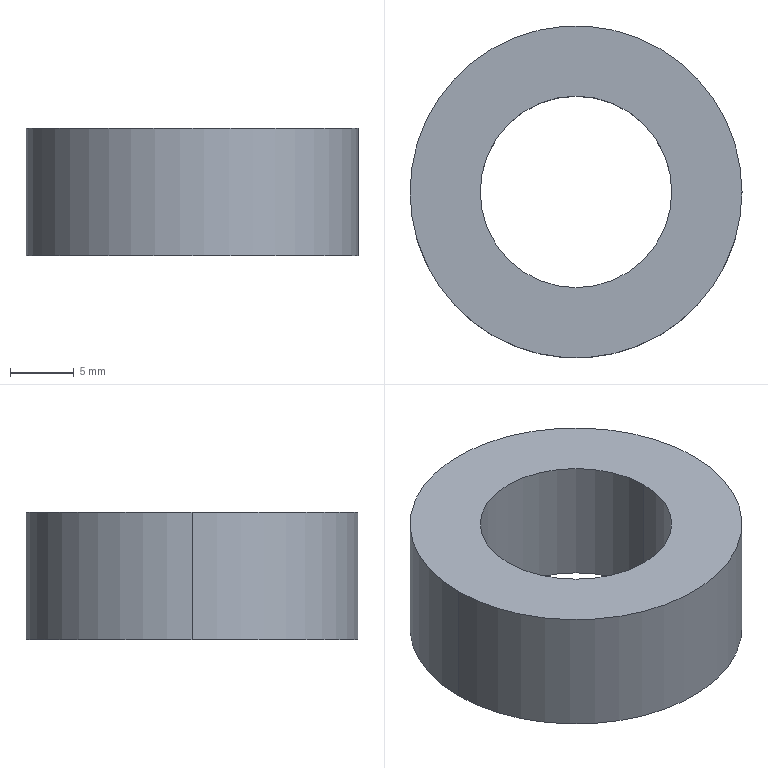Part | SolidWorks | features Extrusion 1 | 1 solid | 6 faces | box 26 x 26 x 10 mm | volume 3542 mm3 | cylinder 4 | plane 2 | commonest cylinder face diameters 15 x2 26 x2
STEP:
#1=CARTESIAN_POINT('',(-7.5,0.,5.));
#2=VERTEX_POINT('',#1);
#3=CARTESIAN_POINT('',(7.5,0.,5.));
#4=VERTEX_POINT('',#3);
#5=CARTESIAN_POINT('',(0.,0.,5.));
#6=DIRECTION('',(0.,0.,1.));
#7=DIRECTION('',(1.,0.,0.));
#8=AXIS2_PLACEMENT_3D('',#5,#6,#7);
#9=CIRCLE('',#8,7.5);
#10=EDGE_CURVE('',#2,#4,#9,.T.);
#11=ORIENTED_EDGE('',*,*,#10,.T.);
#12=CARTESIAN_POINT('',(7.5,0.,-5.));
#13=VERTEX_POINT('',#12);
#14=CARTESIAN_POINT('',(7.5,0.,5.));
#15=DIRECTION('',(0.,0.,-1.));
#16=VECTOR('',#15,1000.);
#17=LINE('',#14,#16);
#18=EDGE_CURVE('',#4,#13,#17,.T.);
#19=ORIENTED_EDGE('',*,*,#18,.T.);
#20=CARTESIAN_POINT('',(-7.5,0.,-5.));
#21=VERTEX_POINT('',#20);
#22=CARTESIAN_POINT('',(0.,0.,-5.));
#23=DIRECTION('',(0.,0.,1.));
#24=DIRECTION('',(1.,0.,0.));
#25=AXIS2_PLACEMENT_3D('',#22,#23,#24);
#26=CIRCLE('',#25,7.5);
#27=EDGE_CURVE('',#21,#13,#26,.T.);
#28=ORIENTED_EDGE('',*,*,#27,.F.);
#29=CARTESIAN_POINT('',(-7.5,0.,5.));
#30=DIRECTION('',(0.,0.,-1.));
#31=VECTOR('',#30,1000.);
#32=LINE('',#29,#31);
#33=EDGE_CURVE('',#2,#21,#32,.T.);
#34=ORIENTED_EDGE('',*,*,#33,.F.);
#35=EDGE_LOOP('',(#11,#19,#28,#34));
#36=FACE_OUTER_BOUND('',#35,.T.);
#37=CARTESIAN_POINT('',(0.,0.,5.));
#38=DIRECTION('',(0.,0.,-1.));
#39=DIRECTION('',(-1.,0.,0.));
#40=AXIS2_PLACEMENT_3D('',#37,#38,#39);
#41=CYLINDRICAL_SURFACE('',#40,7.5);
#42=ADVANCED_FACE('',(#36),#41,.F.);
#43=CARTESIAN_POINT('',(13.,0.,5.));
#44=VERTEX_POINT('',#43);
#45=CARTESIAN_POINT('',(-13.,0.,5.));
#46=VERTEX_POINT('',#45);
#47=CARTESIAN_POINT('',(0.,0.,5.));
#48=DIRECTION('',(0.,0.,1.));
#49=DIRECTION('',(1.,0.,0.));
#50=AXIS2_PLACEMENT_3D('',#47,#48,#49);
#51=CIRCLE('',#50,13.);
#52=EDGE_CURVE('',#44,#46,#51,.T.);
#53=ORIENTED_EDGE('',*,*,#52,.F.);
#54=CARTESIAN_POINT('',(13.,0.,-5.));
#55=VERTEX_POINT('',#54);
#56=CARTESIAN_POINT('',(13.,0.,5.));
#57=DIRECTION('',(0.,0.,-1.));
#58=VECTOR('',#57,1000.);
#59=LINE('',#56,#58);
#60=EDGE_CURVE('',#44,#55,#59,.T.);
#61=ORIENTED_EDGE('',*,*,#60,.T.);
#62=CARTESIAN_POINT('',(-13.,0.,-5.));
#63=VERTEX_POINT('',#62);
#64=CARTESIAN_POINT('',(0.,0.,-5.));
#65=DIRECTION('',(0.,0.,1.));
#66=DIRECTION('',(1.,0.,0.));
#67=AXIS2_PLACEMENT_3D('',#64,#65,#66);
#68=CIRCLE('',#67,13.);
#69=EDGE_CURVE('',#55,#63,#68,.T.);
#70=ORIENTED_EDGE('',*,*,#69,.T.);
#71=CARTESIAN_POINT('',(-13.,0.,5.));
#72=DIRECTION('',(0.,0.,-1.));
#73=VECTOR('',#72,1000.);
#74=LINE('',#71,#73);
#75=EDGE_CURVE('',#46,#63,#74,.T.);
#76=ORIENTED_EDGE('',*,*,#75,.F.);
#77=EDGE_LOOP('',(#53,#61,#70,#76));
#78=FACE_OUTER_BOUND('',#77,.T.);
#79=CARTESIAN_POINT('',(0.,0.,5.));
#80=DIRECTION('',(0.,0.,-1.));
#81=DIRECTION('',(-1.,0.,0.));
#82=AXIS2_PLACEMENT_3D('',#79,#80,#81);
#83=CYLINDRICAL_SURFACE('',#82,13.);
#84=ADVANCED_FACE('',(#78),#83,.T.);
#85=CARTESIAN_POINT('',(0.,0.,5.));
#86=DIRECTION('',(0.,0.,1.));
#87=DIRECTION('',(1.,0.,0.));
#88=AXIS2_PLACEMENT_3D('',#85,#86,#87);
#89=CIRCLE('',#88,13.);
#90=EDGE_CURVE('',#46,#44,#89,.T.);
#91=ORIENTED_EDGE('',*,*,#90,.T.);
#92=ORIENTED_EDGE('',*,*,#52,.T.);
#93=EDGE_LOOP('',(#91,#92));
#94=FACE_OUTER_BOUND('',#93,.T.);
#95=ORIENTED_EDGE('',*,*,#10,.F.);
#96=CARTESIAN_POINT('',(0.,0.,5.));
#97=DIRECTION('',(0.,0.,1.));
#98=DIRECTION('',(1.,0.,0.));
#99=AXIS2_PLACEMENT_3D('',#96,#97,#98);
#100=CIRCLE('',#99,7.5);
#101=EDGE_CURVE('',#4,#2,#100,.T.);
#102=ORIENTED_EDGE('',*,*,#101,.F.);
#103=EDGE_LOOP('',(#95,#102));
#104=FACE_BOUND('',#103,.T.);
#105=CARTESIAN_POINT('',(0.,0.,5.));
#106=DIRECTION('',(0.,0.,1.));
#107=DIRECTION('',(1.,0.,0.));
#108=AXIS2_PLACEMENT_3D('',#105,#106,#107);
#109=PLANE('',#108);
#110=ADVANCED_FACE('',(#94,#104),#109,.T.);
#111=CARTESIAN_POINT('',(0.,0.,-5.));
#112=DIRECTION('',(0.,0.,1.));
#113=DIRECTION('',(1.,0.,0.));
#114=AXIS2_PLACEMENT_3D('',#111,#112,#113);
#115=CIRCLE('',#114,13.);
#116=EDGE_CURVE('',#63,#55,#115,.T.);
#117=ORIENTED_EDGE('',*,*,#116,.F.);
#118=ORIENTED_EDGE('',*,*,#69,.F.);
#119=EDGE_LOOP('',(#117,#118));
#120=FACE_OUTER_BOUND('',#119,.T.);
#121=ORIENTED_EDGE('',*,*,#27,.T.);
#122=CARTESIAN_POINT('',(0.,0.,-5.));
#123=DIRECTION('',(0.,0.,1.));
#124=DIRECTION('',(1.,0.,0.));
#125=AXIS2_PLACEMENT_3D('',#122,#123,#124);
#126=CIRCLE('',#125,7.5);
#127=EDGE_CURVE('',#13,#21,#126,.T.);
#128=ORIENTED_EDGE('',*,*,#127,.T.);
#129=EDGE_LOOP('',(#121,#128));
#130=FACE_BOUND('',#129,.T.);
#131=CARTESIAN_POINT('',(0.,0.,-5.));
#132=DIRECTION('',(0.,0.,1.));
#133=DIRECTION('',(1.,0.,0.));
#134=AXIS2_PLACEMENT_3D('',#131,#132,#133);
#135=PLANE('',#134);
#136=ADVANCED_FACE('',(#120,#130),#135,.F.);
#137=ORIENTED_EDGE('',*,*,#60,.F.);
#138=ORIENTED_EDGE('',*,*,#90,.F.);
#139=ORIENTED_EDGE('',*,*,#75,.T.);
#140=ORIENTED_EDGE('',*,*,#116,.T.);
#141=EDGE_LOOP('',(#137,#138,#139,#140));
#142=FACE_OUTER_BOUND('',#141,.T.);
#143=CARTESIAN_POINT('',(0.,0.,5.));
#144=DIRECTION('',(0.,0.,-1.));
#145=DIRECTION('',(-1.,0.,0.));
#146=AXIS2_PLACEMENT_3D('',#143,#144,#145);
#147=CYLINDRICAL_SURFACE('',#146,13.);
#148=ADVANCED_FACE('',(#142),#147,.T.);
#149=ORIENTED_EDGE('',*,*,#18,.F.);
#150=ORIENTED_EDGE('',*,*,#101,.T.);
#151=ORIENTED_EDGE('',*,*,#33,.T.);
#152=ORIENTED_EDGE('',*,*,#127,.F.);
#153=EDGE_LOOP('',(#149,#150,#151,#152));
#154=FACE_OUTER_BOUND('',#153,.T.);
#155=CARTESIAN_POINT('',(0.,0.,5.));
#156=DIRECTION('',(0.,0.,-1.));
#157=DIRECTION('',(-1.,0.,0.));
#158=AXIS2_PLACEMENT_3D('',#155,#156,#157);
#159=CYLINDRICAL_SURFACE('',#158,7.5);
#160=ADVANCED_FACE('',(#154),#159,.F.);
#161=CLOSED_SHELL('',(#42,#84,#110,#136,#148,#160));
#162=MANIFOLD_SOLID_BREP('',#161);
#163=CARTESIAN_POINT('',(0.,0.,0.));
#164=DIRECTION('',(0.,0.,1.));
#165=DIRECTION('',(1.,0.,0.));
#166=AXIS2_PLACEMENT_3D('',#163,#164,#165);
#167=(LENGTH_UNIT()NAMED_UNIT(*)SI_UNIT(.MILLI.,.METRE.));
#168=UNCERTAINTY_MEASURE_WITH_UNIT(LENGTH_MEASURE(0.00001),#167,'','');
#169=(NAMED_UNIT(*)PLANE_ANGLE_UNIT()SI_UNIT($,.RADIAN.));
#170=(NAMED_UNIT(*)SI_UNIT($,.STERADIAN.)SOLID_ANGLE_UNIT());
#171=(GEOMETRIC_REPRESENTATION_CONTEXT(3)GLOBAL_UNCERTAINTY_ASSIGNED_CONTEXT((#168))GLOBAL_UNIT_ASSIGNED_CONTEXT((#167,#169,#170))REPRESENTATION_CONTEXT('',''));
#172=ADVANCED_BREP_SHAPE_REPRESENTATION('',(#162,#166),#171);